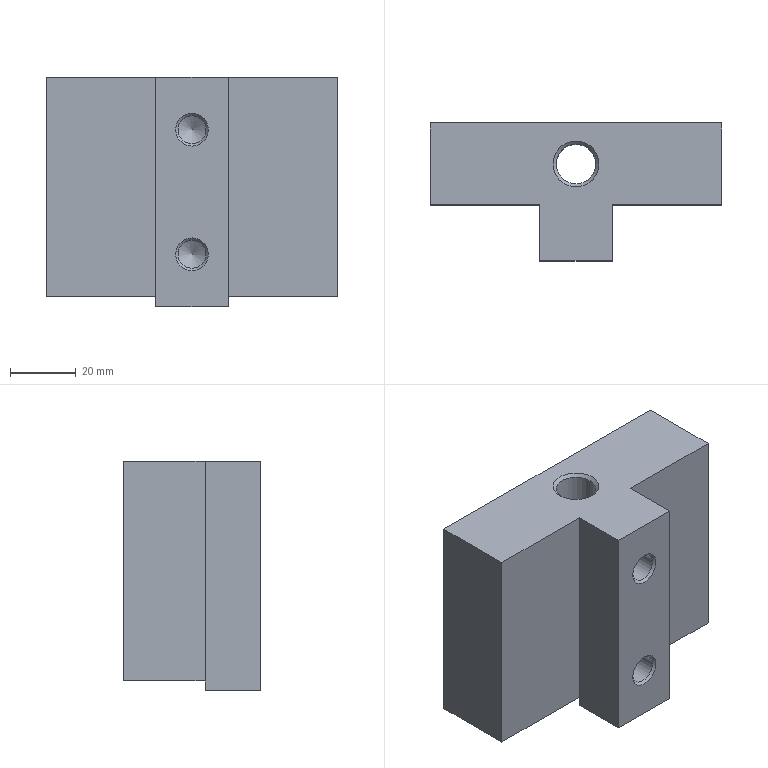Part | NX | features DATUM_CSYS 6, SIMPLE HOLE 5, SKETCH 5, SYMBOLIC_THREAD 5, HOLE PACKAGE 4, EXTRUDE 2 | 1 solid | 27 faces | box 89 x 42 x 70 mm | volume 164920 mm3 | plane 12 | cone 10 | cylinder 5 | commonest cylinder face diameters 3.3 x2 8.5 x2 12.1 x1
STEP:
#1=CARTESIAN_POINT('',(0.,17.,67.));
#2=VERTEX_POINT('',#1);
#3=CARTESIAN_POINT('',(0.,17.,0.));
#4=VERTEX_POINT('',#3);
#5=CARTESIAN_POINT('',(0.,17.,67.));
#6=DIRECTION('',(0.,0.,-1.));
#7=VECTOR('',#6,1000.);
#8=LINE('',#5,#7);
#9=EDGE_CURVE('',#2,#4,#8,.T.);
#10=ORIENTED_EDGE('',*,*,#9,.F.);
#11=CARTESIAN_POINT('',(-33.5,17.,67.));
#12=VERTEX_POINT('',#11);
#13=CARTESIAN_POINT('',(-33.5,17.,67.));
#14=DIRECTION('',(1.,0.,0.));
#15=VECTOR('',#14,1000.);
#16=LINE('',#13,#15);
#17=EDGE_CURVE('',#12,#2,#16,.T.);
#18=ORIENTED_EDGE('',*,*,#17,.F.);
#19=CARTESIAN_POINT('',(-33.5,17.,0.));
#20=VERTEX_POINT('',#19);
#21=CARTESIAN_POINT('',(-33.5,17.,67.));
#22=DIRECTION('',(0.,0.,-1.));
#23=VECTOR('',#22,1000.);
#24=LINE('',#21,#23);
#25=EDGE_CURVE('',#12,#20,#24,.T.);
#26=ORIENTED_EDGE('',*,*,#25,.T.);
#27=CARTESIAN_POINT('',(22.,17.,0.));
#28=DIRECTION('',(1.,0.,0.));
#29=VECTOR('',#28,1000.);
#30=LINE('',#27,#29);
#31=EDGE_CURVE('',#20,#4,#30,.T.);
#32=ORIENTED_EDGE('',*,*,#31,.T.);
#33=EDGE_LOOP('',(#10,#18,#26,#32));
#34=FACE_BOUND('',#33,.T.);
#35=CARTESIAN_POINT('',(22.,17.,67.));
#36=DIRECTION('',(0.,1.,0.));
#37=DIRECTION('',(0.,0.,1.));
#38=AXIS2_PLACEMENT_3D('',#35,#36,#37);
#39=PLANE('',#38);
#40=ADVANCED_FACE('',(#34),#39,.F.);
#41=CARTESIAN_POINT('',(-33.5,42.,0.));
#42=VERTEX_POINT('',#41);
#43=CARTESIAN_POINT('',(-33.5,42.,0.));
#44=DIRECTION('',(0.,-1.,0.));
#45=VECTOR('',#44,1000.);
#46=LINE('',#43,#45);
#47=EDGE_CURVE('',#42,#20,#46,.T.);
#48=ORIENTED_EDGE('',*,*,#47,.T.);
#49=ORIENTED_EDGE('',*,*,#25,.F.);
#50=CARTESIAN_POINT('',(-33.5,42.,67.));
#51=VERTEX_POINT('',#50);
#52=CARTESIAN_POINT('',(-33.5,42.,67.));
#53=DIRECTION('',(0.,-1.,0.));
#54=VECTOR('',#53,1000.);
#55=LINE('',#52,#54);
#56=EDGE_CURVE('',#51,#12,#55,.T.);
#57=ORIENTED_EDGE('',*,*,#56,.F.);
#58=CARTESIAN_POINT('',(-33.5,42.,67.));
#59=DIRECTION('',(0.,0.,-1.));
#60=VECTOR('',#59,1000.);
#61=LINE('',#58,#60);
#62=EDGE_CURVE('',#51,#42,#61,.T.);
#63=ORIENTED_EDGE('',*,*,#62,.T.);
#64=EDGE_LOOP('',(#48,#49,#57,#63));
#65=FACE_BOUND('',#64,.T.);
#66=CARTESIAN_POINT('',(-33.5,42.,67.));
#67=DIRECTION('',(1.,0.,0.));
#68=DIRECTION('',(0.,0.,-1.));
#69=AXIS2_PLACEMENT_3D('',#66,#67,#68);
#70=PLANE('',#69);
#71=ADVANCED_FACE('',(#65),#70,.F.);
#72=CARTESIAN_POINT('',(22.,17.,67.));
#73=VERTEX_POINT('',#72);
#74=CARTESIAN_POINT('',(55.5,17.,67.));
#75=VERTEX_POINT('',#74);
#76=CARTESIAN_POINT('',(-33.5,17.,67.));
#77=DIRECTION('',(1.,0.,0.));
#78=VECTOR('',#77,1000.);
#79=LINE('',#76,#78);
#80=EDGE_CURVE('',#73,#75,#79,.T.);
#81=ORIENTED_EDGE('',*,*,#80,.F.);
#82=CARTESIAN_POINT('',(22.,17.,0.));
#83=VERTEX_POINT('',#82);
#84=CARTESIAN_POINT('',(22.,17.,67.));
#85=DIRECTION('',(0.,0.,-1.));
#86=VECTOR('',#85,1000.);
#87=LINE('',#84,#86);
#88=EDGE_CURVE('',#73,#83,#87,.T.);
#89=ORIENTED_EDGE('',*,*,#88,.T.);
#90=CARTESIAN_POINT('',(55.5,17.,0.));
#91=VERTEX_POINT('',#90);
#92=CARTESIAN_POINT('',(22.,17.,0.));
#93=DIRECTION('',(1.,0.,0.));
#94=VECTOR('',#93,1000.);
#95=LINE('',#92,#94);
#96=EDGE_CURVE('',#83,#91,#95,.T.);
#97=ORIENTED_EDGE('',*,*,#96,.T.);
#98=CARTESIAN_POINT('',(55.5,17.,67.));
#99=DIRECTION('',(0.,0.,-1.));
#100=VECTOR('',#99,1000.);
#101=LINE('',#98,#100);
#102=EDGE_CURVE('',#75,#91,#101,.T.);
#103=ORIENTED_EDGE('',*,*,#102,.F.);
#104=EDGE_LOOP('',(#81,#89,#97,#103));
#105=FACE_BOUND('',#104,.T.);
#106=CARTESIAN_POINT('',(22.,17.,67.));
#107=DIRECTION('',(0.,1.,0.));
#108=DIRECTION('',(0.,0.,1.));
#109=AXIS2_PLACEMENT_3D('',#106,#107,#108);
#110=PLANE('',#109);
#111=ADVANCED_FACE('',(#105),#110,.F.);
#112=CARTESIAN_POINT('',(55.5,42.,0.));
#113=VERTEX_POINT('',#112);
#114=CARTESIAN_POINT('',(55.5,17.,0.));
#115=DIRECTION('',(0.,1.,0.));
#116=VECTOR('',#115,1000.);
#117=LINE('',#114,#116);
#118=EDGE_CURVE('',#91,#113,#117,.T.);
#119=ORIENTED_EDGE('',*,*,#118,.T.);
#120=CARTESIAN_POINT('',(55.5,42.,67.));
#121=VERTEX_POINT('',#120);
#122=CARTESIAN_POINT('',(55.5,42.,67.));
#123=DIRECTION('',(0.,0.,-1.));
#124=VECTOR('',#123,1000.);
#125=LINE('',#122,#124);
#126=EDGE_CURVE('',#121,#113,#125,.T.);
#127=ORIENTED_EDGE('',*,*,#126,.F.);
#128=CARTESIAN_POINT('',(55.5,17.,67.));
#129=DIRECTION('',(0.,1.,0.));
#130=VECTOR('',#129,1000.);
#131=LINE('',#128,#130);
#132=EDGE_CURVE('',#75,#121,#131,.T.);
#133=ORIENTED_EDGE('',*,*,#132,.F.);
#134=ORIENTED_EDGE('',*,*,#102,.T.);
#135=EDGE_LOOP('',(#119,#127,#133,#134));
#136=FACE_BOUND('',#135,.T.);
#137=CARTESIAN_POINT('',(55.5,17.,67.));
#138=DIRECTION('',(-1.,0.,0.));
#139=DIRECTION('',(0.,0.,1.));
#140=AXIS2_PLACEMENT_3D('',#137,#138,#139);
#141=PLANE('',#140);
#142=ADVANCED_FACE('',(#136),#141,.F.);
#143=CARTESIAN_POINT('',(55.5,42.,0.));
#144=DIRECTION('',(-1.,0.,0.));
#145=VECTOR('',#144,1000.);
#146=LINE('',#143,#145);
#147=EDGE_CURVE('',#113,#42,#146,.T.);
#148=ORIENTED_EDGE('',*,*,#147,.T.);
#149=ORIENTED_EDGE('',*,*,#62,.F.);
#150=CARTESIAN_POINT('',(55.5,42.,67.));
#151=DIRECTION('',(-1.,0.,0.));
#152=VECTOR('',#151,1000.);
#153=LINE('',#150,#152);
#154=EDGE_CURVE('',#121,#51,#153,.T.);
#155=ORIENTED_EDGE('',*,*,#154,.F.);
#156=ORIENTED_EDGE('',*,*,#126,.T.);
#157=EDGE_LOOP('',(#148,#149,#155,#156));
#158=FACE_BOUND('',#157,.T.);
#159=CARTESIAN_POINT('',(55.5,42.,67.));
#160=DIRECTION('',(0.,-1.,0.));
#161=DIRECTION('',(0.,0.,-1.));
#162=AXIS2_PLACEMENT_3D('',#159,#160,#161);
#163=PLANE('',#162);
#164=ADVANCED_FACE('',(#158),#163,.F.);
#165=CARTESIAN_POINT('',(18.,29.5,67.));
#166=VERTEX_POINT('',#165);
#167=CARTESIAN_POINT('',(11.,29.5,67.));
#168=DIRECTION('',(0.,0.,1.));
#169=DIRECTION('',(1.,0.,0.));
#170=AXIS2_PLACEMENT_3D('',#167,#168,#169);
#171=CIRCLE('',#170,7.);
#172=EDGE_CURVE('',#166,#166,#171,.F.);
#173=ORIENTED_EDGE('',*,*,#172,.T.);
#174=EDGE_LOOP('',(#173));
#175=FACE_BOUND('',#174,.T.);
#176=ORIENTED_EDGE('',*,*,#56,.T.);
#177=ORIENTED_EDGE('',*,*,#17,.T.);
#178=CARTESIAN_POINT('',(0.,0.,67.));
#179=VERTEX_POINT('',#178);
#180=CARTESIAN_POINT('',(0.,17.,67.));
#181=DIRECTION('',(0.,-1.,0.));
#182=VECTOR('',#181,1000.);
#183=LINE('',#180,#182);
#184=EDGE_CURVE('',#2,#179,#183,.T.);
#185=ORIENTED_EDGE('',*,*,#184,.T.);
#186=CARTESIAN_POINT('',(22.,0.,67.));
#187=VERTEX_POINT('',#186);
#188=CARTESIAN_POINT('',(0.,0.,67.));
#189=DIRECTION('',(1.,0.,0.));
#190=VECTOR('',#189,1000.);
#191=LINE('',#188,#190);
#192=EDGE_CURVE('',#179,#187,#191,.T.);
#193=ORIENTED_EDGE('',*,*,#192,.T.);
#194=CARTESIAN_POINT('',(22.,0.,67.));
#195=DIRECTION('',(0.,1.,0.));
#196=VECTOR('',#195,1000.);
#197=LINE('',#194,#196);
#198=EDGE_CURVE('',#187,#73,#197,.T.);
#199=ORIENTED_EDGE('',*,*,#198,.T.);
#200=ORIENTED_EDGE('',*,*,#80,.T.);
#201=ORIENTED_EDGE('',*,*,#132,.T.);
#202=ORIENTED_EDGE('',*,*,#154,.T.);
#203=EDGE_LOOP('',(#176,#177,#185,#193,#199,#200,#201,#202));
#204=FACE_BOUND('',#203,.T.);
#205=CARTESIAN_POINT('',(0.,0.,67.));
#206=DIRECTION('',(0.,0.,1.));
#207=DIRECTION('',(1.,0.,0.));
#208=AXIS2_PLACEMENT_3D('',#205,#206,#207);
#209=PLANE('',#208);
#210=ADVANCED_FACE('',(#175,#204),#209,.T.);
#211=CARTESIAN_POINT('',(18.,29.5,0.));
#212=VERTEX_POINT('',#211);
#213=CARTESIAN_POINT('',(11.,29.5,0.));
#214=DIRECTION('',(0.,0.,1.));
#215=DIRECTION('',(1.,0.,0.));
#216=AXIS2_PLACEMENT_3D('',#213,#214,#215);
#217=CIRCLE('',#216,7.);
#218=EDGE_CURVE('',#212,#212,#217,.T.);
#219=ORIENTED_EDGE('',*,*,#218,.T.);
#220=EDGE_LOOP('',(#219));
#221=FACE_BOUND('',#220,.T.);
#222=CARTESIAN_POINT('',(43.412,29.5,0.));
#223=VERTEX_POINT('',#222);
#224=CARTESIAN_POINT('',(41.412,29.5,0.));
#225=DIRECTION('',(0.,0.,1.));
#226=DIRECTION('',(1.,0.,0.));
#227=AXIS2_PLACEMENT_3D('',#224,#225,#226);
#228=CIRCLE('',#227,2.);
#229=EDGE_CURVE('',#223,#223,#228,.T.);
#230=ORIENTED_EDGE('',*,*,#229,.T.);
#231=EDGE_LOOP('',(#230));
#232=FACE_BOUND('',#231,.T.);
#233=CARTESIAN_POINT('',(-17.412,29.5,0.));
#234=VERTEX_POINT('',#233);
#235=CARTESIAN_POINT('',(-19.412,29.5,0.));
#236=DIRECTION('',(0.,0.,1.));
#237=DIRECTION('',(1.,0.,0.));
#238=AXIS2_PLACEMENT_3D('',#235,#236,#237);
#239=CIRCLE('',#238,2.);
#240=EDGE_CURVE('',#234,#234,#239,.T.);
#241=ORIENTED_EDGE('',*,*,#240,.T.);
#242=EDGE_LOOP('',(#241));
#243=FACE_BOUND('',#242,.T.);
#244=ORIENTED_EDGE('',*,*,#47,.F.);
#245=ORIENTED_EDGE('',*,*,#147,.F.);
#246=ORIENTED_EDGE('',*,*,#118,.F.);
#247=ORIENTED_EDGE('',*,*,#96,.F.);
#248=CARTESIAN_POINT('',(22.,17.,0.));
#249=DIRECTION('',(1.,0.,0.));
#250=VECTOR('',#249,1000.);
#251=LINE('',#248,#250);
#252=EDGE_CURVE('',#4,#83,#251,.T.);
#253=ORIENTED_EDGE('',*,*,#252,.F.);
#254=ORIENTED_EDGE('',*,*,#31,.F.);
#255=EDGE_LOOP('',(#244,#245,#246,#247,#253,#254));
#256=FACE_BOUND('',#255,.T.);
#257=CARTESIAN_POINT('',(0.,0.,0.));
#258=DIRECTION('',(0.,0.,1.));
#259=DIRECTION('',(1.,0.,0.));
#260=AXIS2_PLACEMENT_3D('',#257,#258,#259);
#261=PLANE('',#260);
#262=ADVANCED_FACE('',(#221,#232,#243,#256),#261,.F.);
#263=CARTESIAN_POINT('',(0.,17.,-3.));
#264=VERTEX_POINT('',#263);
#265=CARTESIAN_POINT('',(0.,17.,67.));
#266=DIRECTION('',(0.,0.,-1.));
#267=VECTOR('',#266,1000.);
#268=LINE('',#265,#267);
#269=EDGE_CURVE('',#4,#264,#268,.T.);
#270=ORIENTED_EDGE('',*,*,#269,.F.);
#271=ORIENTED_EDGE('',*,*,#252,.T.);
#272=CARTESIAN_POINT('',(22.,17.,-3.));
#273=VERTEX_POINT('',#272);
#274=CARTESIAN_POINT('',(22.,17.,67.));
#275=DIRECTION('',(0.,0.,-1.));
#276=VECTOR('',#275,1000.);
#277=LINE('',#274,#276);
#278=EDGE_CURVE('',#83,#273,#277,.T.);
#279=ORIENTED_EDGE('',*,*,#278,.T.);
#280=CARTESIAN_POINT('',(22.,17.,-3.));
#281=DIRECTION('',(-1.,0.,0.));
#282=VECTOR('',#281,1000.);
#283=LINE('',#280,#282);
#284=EDGE_CURVE('',#273,#264,#283,.T.);
#285=ORIENTED_EDGE('',*,*,#284,.T.);
#286=EDGE_LOOP('',(#270,#271,#279,#285));
#287=FACE_BOUND('',#286,.T.);
#288=CARTESIAN_POINT('',(22.,17.,67.));
#289=DIRECTION('',(0.,-1.,0.));
#290=DIRECTION('',(1.,0.,0.));
#291=AXIS2_PLACEMENT_3D('',#288,#289,#290);
#292=PLANE('',#291);
#293=ADVANCED_FACE('',(#287),#292,.F.);
#294=CARTESIAN_POINT('',(0.,0.,-3.));
#295=VERTEX_POINT('',#294);
#296=CARTESIAN_POINT('',(0.,17.,-3.));
#297=DIRECTION('',(0.,-1.,0.));
#298=VECTOR('',#297,1000.);
#299=LINE('',#296,#298);
#300=EDGE_CURVE('',#264,#295,#299,.T.);
#301=ORIENTED_EDGE('',*,*,#300,.T.);
#302=CARTESIAN_POINT('',(0.,0.,67.));
#303=DIRECTION('',(0.,0.,-1.));
#304=VECTOR('',#303,1000.);
#305=LINE('',#302,#304);
#306=EDGE_CURVE('',#179,#295,#305,.T.);
#307=ORIENTED_EDGE('',*,*,#306,.F.);
#308=ORIENTED_EDGE('',*,*,#184,.F.);
#309=ORIENTED_EDGE('',*,*,#9,.T.);
#310=ORIENTED_EDGE('',*,*,#269,.T.);
#311=EDGE_LOOP('',(#301,#307,#308,#309,#310));
#312=FACE_BOUND('',#311,.T.);
#313=CARTESIAN_POINT('',(0.,17.,67.));
#314=DIRECTION('',(1.,0.,0.));
#315=DIRECTION('',(0.,0.,-1.));
#316=AXIS2_PLACEMENT_3D('',#313,#314,#315);
#317=PLANE('',#316);
#318=ADVANCED_FACE('',(#312),#317,.F.);
#319=CARTESIAN_POINT('',(11.,0.,18.));
#320=VERTEX_POINT('',#319);
#321=CARTESIAN_POINT('',(11.,0.,13.));
#322=DIRECTION('',(0.,1.,0.));
#323=DIRECTION('',(0.,0.,1.));
#324=AXIS2_PLACEMENT_3D('',#321,#322,#323);
#325=CIRCLE('',#324,5.);
#326=EDGE_CURVE('',#320,#320,#325,.T.);
#327=ORIENTED_EDGE('',*,*,#326,.T.);
#328=EDGE_LOOP('',(#327));
#329=FACE_BOUND('',#328,.T.);
#330=CARTESIAN_POINT('',(11.,0.,56.));
#331=VERTEX_POINT('',#330);
#332=CARTESIAN_POINT('',(11.,0.,51.));
#333=DIRECTION('',(0.,1.,0.));
#334=DIRECTION('',(0.,0.,1.));
#335=AXIS2_PLACEMENT_3D('',#332,#333,#334);
#336=CIRCLE('',#335,5.);
#337=EDGE_CURVE('',#331,#331,#336,.T.);
#338=ORIENTED_EDGE('',*,*,#337,.T.);
#339=EDGE_LOOP('',(#338));
#340=FACE_BOUND('',#339,.T.);
#341=CARTESIAN_POINT('',(22.,0.,-3.));
#342=VERTEX_POINT('',#341);
#343=CARTESIAN_POINT('',(0.,0.,-3.));
#344=DIRECTION('',(1.,0.,0.));
#345=VECTOR('',#344,1000.);
#346=LINE('',#343,#345);
#347=EDGE_CURVE('',#295,#342,#346,.T.);
#348=ORIENTED_EDGE('',*,*,#347,.T.);
#349=CARTESIAN_POINT('',(22.,0.,67.));
#350=DIRECTION('',(0.,0.,-1.));
#351=VECTOR('',#350,1000.);
#352=LINE('',#349,#351);
#353=EDGE_CURVE('',#187,#342,#352,.T.);
#354=ORIENTED_EDGE('',*,*,#353,.F.);
#355=ORIENTED_EDGE('',*,*,#192,.F.);
#356=ORIENTED_EDGE('',*,*,#306,.T.);
#357=EDGE_LOOP('',(#348,#354,#355,#356));
#358=FACE_BOUND('',#357,.T.);
#359=CARTESIAN_POINT('',(0.,0.,67.));
#360=DIRECTION('',(0.,1.,0.));
#361=DIRECTION('',(0.,0.,1.));
#362=AXIS2_PLACEMENT_3D('',#359,#360,#361);
#363=PLANE('',#362);
#364=ADVANCED_FACE('',(#329,#340,#358),#363,.F.);
#365=CARTESIAN_POINT('',(22.,0.,-3.));
#366=DIRECTION('',(0.,1.,0.));
#367=VECTOR('',#366,1000.);
#368=LINE('',#365,#367);
#369=EDGE_CURVE('',#342,#273,#368,.T.);
#370=ORIENTED_EDGE('',*,*,#369,.T.);
#371=ORIENTED_EDGE('',*,*,#278,.F.);
#372=ORIENTED_EDGE('',*,*,#88,.F.);
#373=ORIENTED_EDGE('',*,*,#198,.F.);
#374=ORIENTED_EDGE('',*,*,#353,.T.);
#375=EDGE_LOOP('',(#370,#371,#372,#373,#374));
#376=FACE_BOUND('',#375,.T.);
#377=CARTESIAN_POINT('',(22.,0.,67.));
#378=DIRECTION('',(-1.,0.,0.));
#379=DIRECTION('',(0.,-1.,0.));
#380=AXIS2_PLACEMENT_3D('',#377,#378,#379);
#381=PLANE('',#380);
#382=ADVANCED_FACE('',(#376),#381,.F.);
#383=ORIENTED_EDGE('',*,*,#300,.F.);
#384=ORIENTED_EDGE('',*,*,#284,.F.);
#385=ORIENTED_EDGE('',*,*,#369,.F.);
#386=ORIENTED_EDGE('',*,*,#347,.F.);
#387=EDGE_LOOP('',(#383,#384,#385,#386));
#388=FACE_BOUND('',#387,.T.);
#389=CARTESIAN_POINT('',(0.,0.,-3.));
#390=DIRECTION('',(0.,0.,1.));
#391=DIRECTION('',(1.,0.,0.));
#392=AXIS2_PLACEMENT_3D('',#389,#390,#391);
#393=PLANE('',#392);
#394=ADVANCED_FACE('',(#388),#393,.F.);
#395=CARTESIAN_POINT('',(-17.762,29.5,12.));
#396=VERTEX_POINT('',#395);
#397=CARTESIAN_POINT('',(-19.412,29.5,12.));
#398=DIRECTION('',(0.,0.,1.));
#399=DIRECTION('',(1.,0.,0.));
#400=AXIS2_PLACEMENT_3D('',#397,#398,#399);
#401=CIRCLE('',#400,1.65);
#402=EDGE_CURVE('',#396,#396,#401,.F.);
#403=ORIENTED_EDGE('',*,*,#402,.T.);
#404=EDGE_LOOP('',(#403));
#405=FACE_BOUND('',#404,.T.);
#406=CARTESIAN_POINT('',(-19.412,29.5,12.991));
#407=VERTEX_POINT('',#406);
#408=VERTEX_LOOP('',#407);
#409=FACE_BOUND('',#408,.T.);
#410=CARTESIAN_POINT('',(-19.412,29.5,12.));
#411=DIRECTION('',(0.,0.,-1.));
#412=DIRECTION('',(-1.,0.,0.));
#413=AXIS2_PLACEMENT_3D('',#410,#411,#412);
#414=CONICAL_SURFACE('',#413,1.65,1.03);
#415=ADVANCED_FACE('',(#405,#409),#414,.F.);
#416=CARTESIAN_POINT('',(-17.762,29.5,0.35));
#417=VERTEX_POINT('',#416);
#418=CARTESIAN_POINT('',(-19.412,29.5,0.35));
#419=DIRECTION('',(0.,0.,1.));
#420=DIRECTION('',(1.,0.,0.));
#421=AXIS2_PLACEMENT_3D('',#418,#419,#420);
#422=CIRCLE('',#421,1.65);
#423=EDGE_CURVE('',#417,#417,#422,.F.);
#424=ORIENTED_EDGE('',*,*,#423,.T.);
#425=EDGE_LOOP('',(#424));
#426=FACE_BOUND('',#425,.T.);
#427=ORIENTED_EDGE('',*,*,#402,.F.);
#428=EDGE_LOOP('',(#427));
#429=FACE_BOUND('',#428,.T.);
#430=CARTESIAN_POINT('',(-19.412,29.5,0.));
#431=DIRECTION('',(0.,0.,1.));
#432=DIRECTION('',(1.,0.,0.));
#433=AXIS2_PLACEMENT_3D('',#430,#431,#432);
#434=CYLINDRICAL_SURFACE('',#433,1.65);
#435=ADVANCED_FACE('',(#426,#429),#434,.F.);
#436=ORIENTED_EDGE('',*,*,#423,.F.);
#437=EDGE_LOOP('',(#436));
#438=FACE_BOUND('',#437,.T.);
#439=ORIENTED_EDGE('',*,*,#240,.F.);
#440=EDGE_LOOP('',(#439));
#441=FACE_BOUND('',#440,.T.);
#442=CARTESIAN_POINT('',(-19.412,29.5,0.));
#443=DIRECTION('',(0.,0.,-1.));
#444=DIRECTION('',(-1.,0.,0.));
#445=AXIS2_PLACEMENT_3D('',#442,#443,#444);
#446=CONICAL_SURFACE('',#445,2.,0.7854);
#447=ADVANCED_FACE('',(#438,#441),#446,.F.);
#448=CARTESIAN_POINT('',(43.062,29.5,12.));
#449=VERTEX_POINT('',#448);
#450=CARTESIAN_POINT('',(41.412,29.5,12.));
#451=DIRECTION('',(0.,0.,1.));
#452=DIRECTION('',(1.,0.,0.));
#453=AXIS2_PLACEMENT_3D('',#450,#451,#452);
#454=CIRCLE('',#453,1.65);
#455=EDGE_CURVE('',#449,#449,#454,.F.);
#456=ORIENTED_EDGE('',*,*,#455,.T.);
#457=EDGE_LOOP('',(#456));
#458=FACE_BOUND('',#457,.T.);
#459=CARTESIAN_POINT('',(41.412,29.5,12.991));
#460=VERTEX_POINT('',#459);
#461=VERTEX_LOOP('',#460);
#462=FACE_BOUND('',#461,.T.);
#463=CARTESIAN_POINT('',(41.412,29.5,12.));
#464=DIRECTION('',(0.,0.,-1.));
#465=DIRECTION('',(-1.,0.,0.));
#466=AXIS2_PLACEMENT_3D('',#463,#464,#465);
#467=CONICAL_SURFACE('',#466,1.65,1.03);
#468=ADVANCED_FACE('',(#458,#462),#467,.F.);
#469=CARTESIAN_POINT('',(43.062,29.5,0.35));
#470=VERTEX_POINT('',#469);
#471=CARTESIAN_POINT('',(41.412,29.5,0.35));
#472=DIRECTION('',(0.,0.,1.));
#473=DIRECTION('',(1.,0.,0.));
#474=AXIS2_PLACEMENT_3D('',#471,#472,#473);
#475=CIRCLE('',#474,1.65);
#476=EDGE_CURVE('',#470,#470,#475,.F.);
#477=ORIENTED_EDGE('',*,*,#476,.T.);
#478=EDGE_LOOP('',(#477));
#479=FACE_BOUND('',#478,.T.);
#480=ORIENTED_EDGE('',*,*,#455,.F.);
#481=EDGE_LOOP('',(#480));
#482=FACE_BOUND('',#481,.T.);
#483=CARTESIAN_POINT('',(41.412,29.5,0.));
#484=DIRECTION('',(0.,0.,1.));
#485=DIRECTION('',(1.,0.,0.));
#486=AXIS2_PLACEMENT_3D('',#483,#484,#485);
#487=CYLINDRICAL_SURFACE('',#486,1.65);
#488=ADVANCED_FACE('',(#479,#482),#487,.F.);
#489=ORIENTED_EDGE('',*,*,#476,.F.);
#490=EDGE_LOOP('',(#489));
#491=FACE_BOUND('',#490,.T.);
#492=ORIENTED_EDGE('',*,*,#229,.F.);
#493=EDGE_LOOP('',(#492));
#494=FACE_BOUND('',#493,.T.);
#495=CARTESIAN_POINT('',(41.412,29.5,0.));
#496=DIRECTION('',(0.,0.,-1.));
#497=DIRECTION('',(-1.,0.,0.));
#498=AXIS2_PLACEMENT_3D('',#495,#496,#497);
#499=CONICAL_SURFACE('',#498,2.,0.7854);
#500=ADVANCED_FACE('',(#491,#494),#499,.F.);
#501=CARTESIAN_POINT('',(17.05,29.5,66.05));
#502=VERTEX_POINT('',#501);
#503=CARTESIAN_POINT('',(11.,29.5,66.05));
#504=DIRECTION('',(0.,0.,1.));
#505=DIRECTION('',(1.,0.,0.));
#506=AXIS2_PLACEMENT_3D('',#503,#504,#505);
#507=CIRCLE('',#506,6.05);
#508=EDGE_CURVE('',#502,#502,#507,.T.);
#509=ORIENTED_EDGE('',*,*,#508,.T.);
#510=EDGE_LOOP('',(#509));
#511=FACE_BOUND('',#510,.T.);
#512=CARTESIAN_POINT('',(17.05,29.5,0.95));
#513=VERTEX_POINT('',#512);
#514=CARTESIAN_POINT('',(11.,29.5,0.95));
#515=DIRECTION('',(0.,0.,1.));
#516=DIRECTION('',(1.,0.,0.));
#517=AXIS2_PLACEMENT_3D('',#514,#515,#516);
#518=CIRCLE('',#517,6.05);
#519=EDGE_CURVE('',#513,#513,#518,.F.);
#520=ORIENTED_EDGE('',*,*,#519,.T.);
#521=EDGE_LOOP('',(#520));
#522=FACE_BOUND('',#521,.T.);
#523=CARTESIAN_POINT('',(11.,29.5,0.));
#524=DIRECTION('',(0.,0.,1.));
#525=DIRECTION('',(1.,0.,0.));
#526=AXIS2_PLACEMENT_3D('',#523,#524,#525);
#527=CYLINDRICAL_SURFACE('',#526,6.05);
#528=ADVANCED_FACE('',(#511,#522),#527,.F.);
#529=ORIENTED_EDGE('',*,*,#519,.F.);
#530=EDGE_LOOP('',(#529));
#531=FACE_BOUND('',#530,.T.);
#532=ORIENTED_EDGE('',*,*,#218,.F.);
#533=EDGE_LOOP('',(#532));
#534=FACE_BOUND('',#533,.T.);
#535=CARTESIAN_POINT('',(11.,29.5,0.));
#536=DIRECTION('',(0.,0.,-1.));
#537=DIRECTION('',(-1.,0.,0.));
#538=AXIS2_PLACEMENT_3D('',#535,#536,#537);
#539=CONICAL_SURFACE('',#538,7.,0.7854);
#540=ADVANCED_FACE('',(#531,#534),#539,.F.);
#541=ORIENTED_EDGE('',*,*,#172,.F.);
#542=EDGE_LOOP('',(#541));
#543=FACE_BOUND('',#542,.T.);
#544=ORIENTED_EDGE('',*,*,#508,.F.);
#545=EDGE_LOOP('',(#544));
#546=FACE_BOUND('',#545,.T.);
#547=CARTESIAN_POINT('',(11.,29.5,66.05));
#548=DIRECTION('',(0.,0.,1.));
#549=DIRECTION('',(1.,0.,0.));
#550=AXIS2_PLACEMENT_3D('',#547,#548,#549);
#551=CONICAL_SURFACE('',#550,6.05,0.7854);
#552=ADVANCED_FACE('',(#543,#546),#551,.F.);
#553=CARTESIAN_POINT('',(11.,20.,55.25));
#554=VERTEX_POINT('',#553);
#555=CARTESIAN_POINT('',(11.,20.,51.));
#556=DIRECTION('',(0.,1.,0.));
#557=DIRECTION('',(0.,0.,1.));
#558=AXIS2_PLACEMENT_3D('',#555,#556,#557);
#559=CIRCLE('',#558,4.25);
#560=EDGE_CURVE('',#554,#554,#559,.F.);
#561=ORIENTED_EDGE('',*,*,#560,.T.);
#562=EDGE_LOOP('',(#561));
#563=FACE_BOUND('',#562,.T.);
#564=CARTESIAN_POINT('',(11.,22.554,51.));
#565=VERTEX_POINT('',#564);
#566=VERTEX_LOOP('',#565);
#567=FACE_BOUND('',#566,.T.);
#568=CARTESIAN_POINT('',(11.,20.,51.));
#569=DIRECTION('',(0.,-1.,0.));
#570=DIRECTION('',(0.,0.,-1.));
#571=AXIS2_PLACEMENT_3D('',#568,#569,#570);
#572=CONICAL_SURFACE('',#571,4.25,1.03);
#573=ADVANCED_FACE('',(#563,#567),#572,.F.);
#574=CARTESIAN_POINT('',(11.,0.75,55.25));
#575=VERTEX_POINT('',#574);
#576=CARTESIAN_POINT('',(11.,0.75,51.));
#577=DIRECTION('',(0.,1.,0.));
#578=DIRECTION('',(0.,0.,1.));
#579=AXIS2_PLACEMENT_3D('',#576,#577,#578);
#580=CIRCLE('',#579,4.25);
#581=EDGE_CURVE('',#575,#575,#580,.F.);
#582=ORIENTED_EDGE('',*,*,#581,.T.);
#583=EDGE_LOOP('',(#582));
#584=FACE_BOUND('',#583,.T.);
#585=ORIENTED_EDGE('',*,*,#560,.F.);
#586=EDGE_LOOP('',(#585));
#587=FACE_BOUND('',#586,.T.);
#588=CARTESIAN_POINT('',(11.,0.,51.));
#589=DIRECTION('',(0.,1.,0.));
#590=DIRECTION('',(0.,0.,1.));
#591=AXIS2_PLACEMENT_3D('',#588,#589,#590);
#592=CYLINDRICAL_SURFACE('',#591,4.25);
#593=ADVANCED_FACE('',(#584,#587),#592,.F.);
#594=ORIENTED_EDGE('',*,*,#581,.F.);
#595=EDGE_LOOP('',(#594));
#596=FACE_BOUND('',#595,.T.);
#597=ORIENTED_EDGE('',*,*,#337,.F.);
#598=EDGE_LOOP('',(#597));
#599=FACE_BOUND('',#598,.T.);
#600=CARTESIAN_POINT('',(11.,0.,51.));
#601=DIRECTION('',(0.,-1.,0.));
#602=DIRECTION('',(0.,0.,-1.));
#603=AXIS2_PLACEMENT_3D('',#600,#601,#602);
#604=CONICAL_SURFACE('',#603,5.,0.7854);
#605=ADVANCED_FACE('',(#596,#599),#604,.F.);
#606=CARTESIAN_POINT('',(11.,20.,17.25));
#607=VERTEX_POINT('',#606);
#608=CARTESIAN_POINT('',(11.,20.,13.));
#609=DIRECTION('',(0.,1.,0.));
#610=DIRECTION('',(0.,0.,1.));
#611=AXIS2_PLACEMENT_3D('',#608,#609,#610);
#612=CIRCLE('',#611,4.25);
#613=EDGE_CURVE('',#607,#607,#612,.F.);
#614=ORIENTED_EDGE('',*,*,#613,.T.);
#615=EDGE_LOOP('',(#614));
#616=FACE_BOUND('',#615,.T.);
#617=CARTESIAN_POINT('',(11.,22.554,13.));
#618=VERTEX_POINT('',#617);
#619=VERTEX_LOOP('',#618);
#620=FACE_BOUND('',#619,.T.);
#621=CARTESIAN_POINT('',(11.,20.,13.));
#622=DIRECTION('',(0.,-1.,0.));
#623=DIRECTION('',(0.,0.,-1.));
#624=AXIS2_PLACEMENT_3D('',#621,#622,#623);
#625=CONICAL_SURFACE('',#624,4.25,1.03);
#626=ADVANCED_FACE('',(#616,#620),#625,.F.);
#627=CARTESIAN_POINT('',(11.,0.75,17.25));
#628=VERTEX_POINT('',#627);
#629=CARTESIAN_POINT('',(11.,0.75,13.));
#630=DIRECTION('',(0.,1.,0.));
#631=DIRECTION('',(0.,0.,1.));
#632=AXIS2_PLACEMENT_3D('',#629,#630,#631);
#633=CIRCLE('',#632,4.25);
#634=EDGE_CURVE('',#628,#628,#633,.F.);
#635=ORIENTED_EDGE('',*,*,#634,.T.);
#636=EDGE_LOOP('',(#635));
#637=FACE_BOUND('',#636,.T.);
#638=ORIENTED_EDGE('',*,*,#613,.F.);
#639=EDGE_LOOP('',(#638));
#640=FACE_BOUND('',#639,.T.);
#641=CARTESIAN_POINT('',(11.,0.,13.));
#642=DIRECTION('',(0.,1.,0.));
#643=DIRECTION('',(0.,0.,1.));
#644=AXIS2_PLACEMENT_3D('',#641,#642,#643);
#645=CYLINDRICAL_SURFACE('',#644,4.25);
#646=ADVANCED_FACE('',(#637,#640),#645,.F.);
#647=ORIENTED_EDGE('',*,*,#634,.F.);
#648=EDGE_LOOP('',(#647));
#649=FACE_BOUND('',#648,.T.);
#650=ORIENTED_EDGE('',*,*,#326,.F.);
#651=EDGE_LOOP('',(#650));
#652=FACE_BOUND('',#651,.T.);
#653=CARTESIAN_POINT('',(11.,0.,13.));
#654=DIRECTION('',(0.,-1.,0.));
#655=DIRECTION('',(0.,0.,-1.));
#656=AXIS2_PLACEMENT_3D('',#653,#654,#655);
#657=CONICAL_SURFACE('',#656,5.,0.7854);
#658=ADVANCED_FACE('',(#649,#652),#657,.F.);
#659=CLOSED_SHELL('',(#40,#71,#111,#142,#164,#210,#262,#293,#318,#364,#382,#394,#415,#435,#447,#468,#488,#500,#528,#540,#552,#573,#593,#605,#626,#646,#658));
#660=MANIFOLD_SOLID_BREP('',#659);
#661=(LENGTH_UNIT()NAMED_UNIT(*)SI_UNIT(.MILLI.,.METRE.));
#662=UNCERTAINTY_MEASURE_WITH_UNIT(LENGTH_MEASURE(0.00001),#661,'','');
#663=(NAMED_UNIT(*)PLANE_ANGLE_UNIT()SI_UNIT($,.RADIAN.));
#664=(NAMED_UNIT(*)SI_UNIT($,.STERADIAN.)SOLID_ANGLE_UNIT());
#665=(GEOMETRIC_REPRESENTATION_CONTEXT(3)GLOBAL_UNCERTAINTY_ASSIGNED_CONTEXT((#662))GLOBAL_UNIT_ASSIGNED_CONTEXT((#661,#663,#664))REPRESENTATION_CONTEXT('',''));
#666=ADVANCED_BREP_SHAPE_REPRESENTATION('',(#660),#665);